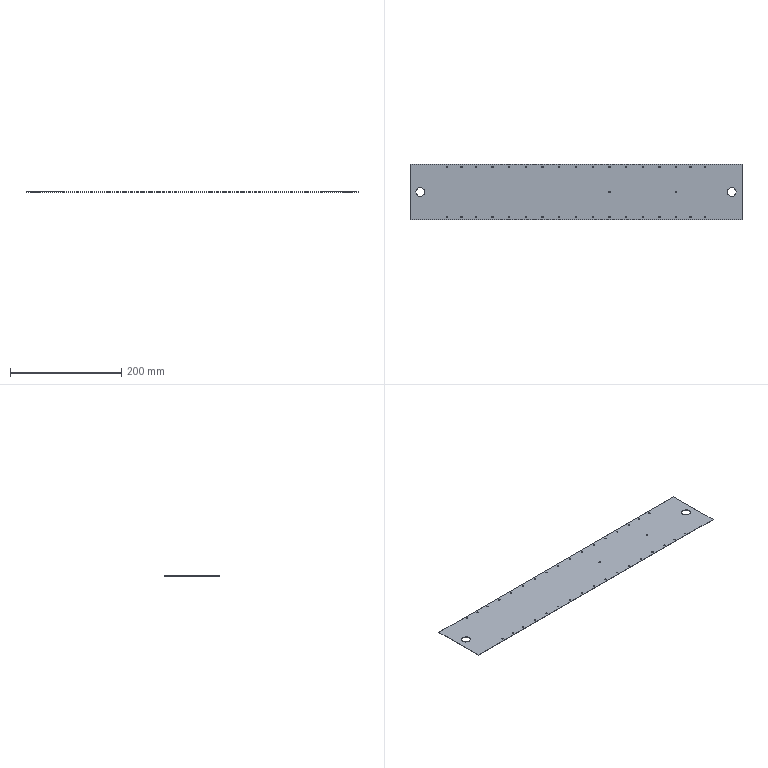Part | SolidWorks | features BaseBody 1 | 1 solid | 82 faces | box 597.2 x 100 x 0.5 mm | volume 29580 mm3 | cylinder 76 | plane 6 | commonest cylinder face diameters 2.4 x72 15.9 x4